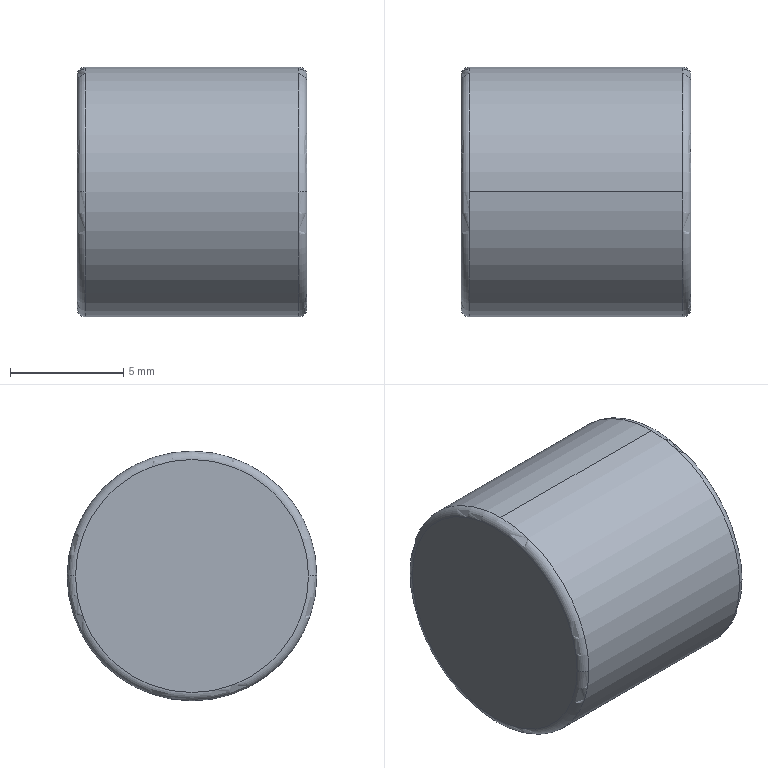Part | SolidWorks | features BaseBody 1 | 1 solid | 8 faces | box 10.125 x 11 x 11 mm | volume 960.225 mm3 | torus 4 | plane 2 | cylinder 2 | commonest cylinder face diameters 11 x2
STEP:
#1=CARTESIAN_POINT('',(-2090.144,780.437,-1577.624));
#2=VERTEX_POINT('',#1);
#3=CARTESIAN_POINT('',(-2090.144,790.7,-1577.624));
#4=VERTEX_POINT('',#3);
#5=CARTESIAN_POINT('',(-2090.144,785.569,-1577.624));
#6=DIRECTION('',(-1.,0.,0.));
#7=DIRECTION('',(0.,0.,1.));
#8=AXIS2_PLACEMENT_3D('',#5,#6,#7);
#9=CIRCLE('',#8,5.131);
#10=EDGE_CURVE('',#2,#4,#9,.T.);
#11=ORIENTED_EDGE('',*,*,#10,.T.);
#12=CARTESIAN_POINT('',(-2090.144,785.569,-1577.624));
#13=DIRECTION('',(-1.,0.,0.));
#14=DIRECTION('',(0.,1.,0.));
#15=AXIS2_PLACEMENT_3D('',#12,#13,#14);
#16=CIRCLE('',#15,5.131);
#17=EDGE_CURVE('',#4,#2,#16,.T.);
#18=ORIENTED_EDGE('',*,*,#17,.T.);
#19=EDGE_LOOP('',(#11,#18));
#20=FACE_OUTER_BOUND('',#19,.T.);
#21=CARTESIAN_POINT('',(-2090.144,779.924,-1583.231));
#22=DIRECTION('',(-1.,0.,0.));
#23=DIRECTION('',(0.,0.,1.));
#24=AXIS2_PLACEMENT_3D('',#21,#22,#23);
#25=PLANE('',#24);
#26=ADVANCED_FACE('',(#20),#25,.T.);
#27=CARTESIAN_POINT('',(-2089.775,780.069,-1577.624));
#28=VERTEX_POINT('',#27);
#29=CARTESIAN_POINT('',(-2089.775,780.437,-1577.624));
#30=DIRECTION('',(0.,0.,-1.));
#31=DIRECTION('',(0.,-1.,0.));
#32=AXIS2_PLACEMENT_3D('',#29,#30,#31);
#33=CIRCLE('',#32,0.3687);
#34=EDGE_CURVE('',#28,#2,#33,.T.);
#35=ORIENTED_EDGE('',*,*,#34,.T.);
#36=ORIENTED_EDGE('',*,*,#17,.F.);
#37=CARTESIAN_POINT('',(-2089.775,791.069,-1577.624));
#38=VERTEX_POINT('',#37);
#39=CARTESIAN_POINT('',(-2089.775,790.7,-1577.624));
#40=DIRECTION('',(0.,0.,-1.));
#41=DIRECTION('',(-1.,0.,0.));
#42=AXIS2_PLACEMENT_3D('',#39,#40,#41);
#43=CIRCLE('',#42,0.3687);
#44=EDGE_CURVE('',#4,#38,#43,.T.);
#45=ORIENTED_EDGE('',*,*,#44,.T.);
#46=CARTESIAN_POINT('',(-2089.775,785.569,-1583.124));
#47=VERTEX_POINT('',#46);
#48=CARTESIAN_POINT('',(-2089.775,785.569,-1577.624));
#49=DIRECTION('',(-1.,0.,0.));
#50=DIRECTION('',(0.,1.,0.));
#51=AXIS2_PLACEMENT_3D('',#48,#49,#50);
#52=CIRCLE('',#51,5.5);
#53=EDGE_CURVE('',#38,#47,#52,.T.);
#54=ORIENTED_EDGE('',*,*,#53,.T.);
#55=CARTESIAN_POINT('',(-2089.775,785.569,-1577.624));
#56=DIRECTION('',(-1.,0.,0.));
#57=DIRECTION('',(0.,0.,-1.));
#58=AXIS2_PLACEMENT_3D('',#55,#56,#57);
#59=CIRCLE('',#58,5.5);
#60=EDGE_CURVE('',#47,#28,#59,.T.);
#61=ORIENTED_EDGE('',*,*,#60,.T.);
#62=EDGE_LOOP('',(#35,#36,#45,#54,#61));
#63=FACE_OUTER_BOUND('',#62,.T.);
#64=CARTESIAN_POINT('',(-2089.775,785.569,-1577.624));
#65=DIRECTION('',(-1.,0.,0.));
#66=DIRECTION('',(0.,0.9962,0.08716));
#67=AXIS2_PLACEMENT_3D('',#64,#65,#66);
#68=TOROIDAL_SURFACE('',#67,5.131,0.3687);
#69=ADVANCED_FACE('',(#63),#68,.T.);
#70=CARTESIAN_POINT('',(-2080.388,785.569,-1572.124));
#71=VERTEX_POINT('',#70);
#72=CARTESIAN_POINT('',(-2089.775,785.569,-1572.124));
#73=VERTEX_POINT('',#72);
#74=CARTESIAN_POINT('',(-2080.388,785.569,-1572.124));
#75=DIRECTION('',(-1.,0.,0.));
#76=VECTOR('',#75,1000.);
#77=LINE('',#74,#76);
#78=EDGE_CURVE('',#71,#73,#77,.T.);
#79=ORIENTED_EDGE('',*,*,#78,.T.);
#80=CARTESIAN_POINT('',(-2089.775,785.569,-1577.624));
#81=DIRECTION('',(-1.,0.,0.));
#82=DIRECTION('',(0.,-1.,0.));
#83=AXIS2_PLACEMENT_3D('',#80,#81,#82);
#84=CIRCLE('',#83,5.5);
#85=EDGE_CURVE('',#28,#73,#84,.T.);
#86=ORIENTED_EDGE('',*,*,#85,.F.);
#87=ORIENTED_EDGE('',*,*,#60,.F.);
#88=CARTESIAN_POINT('',(-2080.388,785.569,-1583.124));
#89=VERTEX_POINT('',#88);
#90=CARTESIAN_POINT('',(-2089.775,785.569,-1583.124));
#91=DIRECTION('',(1.,0.,0.));
#92=VECTOR('',#91,1000.);
#93=LINE('',#90,#92);
#94=EDGE_CURVE('',#47,#89,#93,.T.);
#95=ORIENTED_EDGE('',*,*,#94,.T.);
#96=CARTESIAN_POINT('',(-2080.388,780.069,-1577.624));
#97=VERTEX_POINT('',#96);
#98=CARTESIAN_POINT('',(-2080.388,785.569,-1577.624));
#99=DIRECTION('',(-1.,0.,0.));
#100=DIRECTION('',(0.,0.,-1.));
#101=AXIS2_PLACEMENT_3D('',#98,#99,#100);
#102=CIRCLE('',#101,5.5);
#103=EDGE_CURVE('',#89,#97,#102,.T.);
#104=ORIENTED_EDGE('',*,*,#103,.T.);
#105=CARTESIAN_POINT('',(-2080.388,785.569,-1577.624));
#106=DIRECTION('',(-1.,0.,0.));
#107=DIRECTION('',(0.,-1.,0.));
#108=AXIS2_PLACEMENT_3D('',#105,#106,#107);
#109=CIRCLE('',#108,5.5);
#110=EDGE_CURVE('',#97,#71,#109,.T.);
#111=ORIENTED_EDGE('',*,*,#110,.T.);
#112=EDGE_LOOP('',(#79,#86,#87,#95,#104,#111));
#113=FACE_OUTER_BOUND('',#112,.T.);
#114=CARTESIAN_POINT('',(-2079.919,785.569,-1577.624));
#115=DIRECTION('',(1.,0.,0.));
#116=DIRECTION('',(0.,0.08716,0.9962));
#117=AXIS2_PLACEMENT_3D('',#114,#115,#116);
#118=CYLINDRICAL_SURFACE('',#117,5.5);
#119=ADVANCED_FACE('',(#113),#118,.T.);
#120=CARTESIAN_POINT('',(-2080.019,780.437,-1577.624));
#121=VERTEX_POINT('',#120);
#122=CARTESIAN_POINT('',(-2080.388,780.437,-1577.624));
#123=DIRECTION('',(0.,0.,-1.));
#124=DIRECTION('',(1.,0.,0.));
#125=AXIS2_PLACEMENT_3D('',#122,#123,#124);
#126=CIRCLE('',#125,0.3687);
#127=EDGE_CURVE('',#121,#97,#126,.T.);
#128=ORIENTED_EDGE('',*,*,#127,.T.);
#129=ORIENTED_EDGE('',*,*,#103,.F.);
#130=CARTESIAN_POINT('',(-2080.388,791.069,-1577.624));
#131=VERTEX_POINT('',#130);
#132=CARTESIAN_POINT('',(-2080.388,785.569,-1577.624));
#133=DIRECTION('',(-1.,0.,0.));
#134=DIRECTION('',(0.,1.,0.));
#135=AXIS2_PLACEMENT_3D('',#132,#133,#134);
#136=CIRCLE('',#135,5.5);
#137=EDGE_CURVE('',#131,#89,#136,.T.);
#138=ORIENTED_EDGE('',*,*,#137,.F.);
#139=CARTESIAN_POINT('',(-2080.019,790.7,-1577.624));
#140=VERTEX_POINT('',#139);
#141=CARTESIAN_POINT('',(-2080.388,790.7,-1577.624));
#142=DIRECTION('',(0.,0.,-1.));
#143=DIRECTION('',(0.,1.,0.));
#144=AXIS2_PLACEMENT_3D('',#141,#142,#143);
#145=CIRCLE('',#144,0.3687);
#146=EDGE_CURVE('',#131,#140,#145,.T.);
#147=ORIENTED_EDGE('',*,*,#146,.T.);
#148=CARTESIAN_POINT('',(-2080.019,785.569,-1577.624));
#149=DIRECTION('',(1.,0.,0.));
#150=DIRECTION('',(0.,-1.,0.));
#151=AXIS2_PLACEMENT_3D('',#148,#149,#150);
#152=CIRCLE('',#151,5.131);
#153=EDGE_CURVE('',#121,#140,#152,.T.);
#154=ORIENTED_EDGE('',*,*,#153,.F.);
#155=EDGE_LOOP('',(#128,#129,#138,#147,#154));
#156=FACE_OUTER_BOUND('',#155,.T.);
#157=CARTESIAN_POINT('',(-2080.388,785.569,-1577.624));
#158=DIRECTION('',(-1.,0.,0.));
#159=DIRECTION('',(0.,0.9962,0.08716));
#160=AXIS2_PLACEMENT_3D('',#157,#158,#159);
#161=TOROIDAL_SURFACE('',#160,5.131,0.3687);
#162=ADVANCED_FACE('',(#156),#161,.T.);
#163=CARTESIAN_POINT('',(-2080.019,785.569,-1577.624));
#164=DIRECTION('',(1.,0.,0.));
#165=DIRECTION('',(0.,1.,0.));
#166=AXIS2_PLACEMENT_3D('',#163,#164,#165);
#167=CIRCLE('',#166,5.131);
#168=EDGE_CURVE('',#140,#121,#167,.T.);
#169=ORIENTED_EDGE('',*,*,#168,.T.);
#170=ORIENTED_EDGE('',*,*,#153,.T.);
#171=EDGE_LOOP('',(#169,#170));
#172=FACE_OUTER_BOUND('',#171,.T.);
#173=CARTESIAN_POINT('',(-2080.019,779.924,-1571.98));
#174=DIRECTION('',(1.,0.,0.));
#175=DIRECTION('',(0.,1.,0.));
#176=AXIS2_PLACEMENT_3D('',#173,#174,#175);
#177=PLANE('',#176);
#178=ADVANCED_FACE('',(#172),#177,.T.);
#179=ORIENTED_EDGE('',*,*,#127,.F.);
#180=ORIENTED_EDGE('',*,*,#168,.F.);
#181=ORIENTED_EDGE('',*,*,#146,.F.);
#182=CARTESIAN_POINT('',(-2080.388,785.569,-1577.624));
#183=DIRECTION('',(-1.,0.,0.));
#184=DIRECTION('',(0.,0.,1.));
#185=AXIS2_PLACEMENT_3D('',#182,#183,#184);
#186=CIRCLE('',#185,5.5);
#187=EDGE_CURVE('',#71,#131,#186,.T.);
#188=ORIENTED_EDGE('',*,*,#187,.F.);
#189=ORIENTED_EDGE('',*,*,#110,.F.);
#190=EDGE_LOOP('',(#179,#180,#181,#188,#189));
#191=FACE_OUTER_BOUND('',#190,.T.);
#192=CARTESIAN_POINT('',(-2080.388,785.569,-1577.624));
#193=DIRECTION('',(-1.,0.,0.));
#194=DIRECTION('',(0.,-0.9962,-0.08716));
#195=AXIS2_PLACEMENT_3D('',#192,#193,#194);
#196=TOROIDAL_SURFACE('',#195,5.131,0.3687);
#197=ADVANCED_FACE('',(#191),#196,.T.);
#198=ORIENTED_EDGE('',*,*,#78,.F.);
#199=ORIENTED_EDGE('',*,*,#187,.T.);
#200=ORIENTED_EDGE('',*,*,#137,.T.);
#201=ORIENTED_EDGE('',*,*,#94,.F.);
#202=ORIENTED_EDGE('',*,*,#53,.F.);
#203=CARTESIAN_POINT('',(-2089.775,785.569,-1577.624));
#204=DIRECTION('',(-1.,0.,0.));
#205=DIRECTION('',(0.,0.,1.));
#206=AXIS2_PLACEMENT_3D('',#203,#204,#205);
#207=CIRCLE('',#206,5.5);
#208=EDGE_CURVE('',#73,#38,#207,.T.);
#209=ORIENTED_EDGE('',*,*,#208,.F.);
#210=EDGE_LOOP('',(#198,#199,#200,#201,#202,#209));
#211=FACE_OUTER_BOUND('',#210,.T.);
#212=CARTESIAN_POINT('',(-2079.919,785.569,-1577.624));
#213=DIRECTION('',(1.,0.,0.));
#214=DIRECTION('',(0.,-0.08716,-0.9962));
#215=AXIS2_PLACEMENT_3D('',#212,#213,#214);
#216=CYLINDRICAL_SURFACE('',#215,5.5);
#217=ADVANCED_FACE('',(#211),#216,.T.);
#218=ORIENTED_EDGE('',*,*,#34,.F.);
#219=ORIENTED_EDGE('',*,*,#85,.T.);
#220=ORIENTED_EDGE('',*,*,#208,.T.);
#221=ORIENTED_EDGE('',*,*,#44,.F.);
#222=ORIENTED_EDGE('',*,*,#10,.F.);
#223=EDGE_LOOP('',(#218,#219,#220,#221,#222));
#224=FACE_OUTER_BOUND('',#223,.T.);
#225=CARTESIAN_POINT('',(-2089.775,785.569,-1577.624));
#226=DIRECTION('',(-1.,0.,0.));
#227=DIRECTION('',(0.,-0.9962,-0.08716));
#228=AXIS2_PLACEMENT_3D('',#225,#226,#227);
#229=TOROIDAL_SURFACE('',#228,5.131,0.3687);
#230=ADVANCED_FACE('',(#224),#229,.T.);
#231=CLOSED_SHELL('',(#26,#69,#119,#162,#178,#197,#217,#230));
#232=MANIFOLD_SOLID_BREP('',#231);
#233=CARTESIAN_POINT('',(0.,0.,0.));
#234=DIRECTION('',(0.,0.,1.));
#235=DIRECTION('',(1.,0.,0.));
#236=AXIS2_PLACEMENT_3D('',#233,#234,#235);
#237=(LENGTH_UNIT()NAMED_UNIT(*)SI_UNIT(.MILLI.,.METRE.));
#238=UNCERTAINTY_MEASURE_WITH_UNIT(LENGTH_MEASURE(0.00001),#237,'','');
#239=(NAMED_UNIT(*)PLANE_ANGLE_UNIT()SI_UNIT($,.RADIAN.));
#240=(NAMED_UNIT(*)SI_UNIT($,.STERADIAN.)SOLID_ANGLE_UNIT());
#241=(GEOMETRIC_REPRESENTATION_CONTEXT(3)GLOBAL_UNCERTAINTY_ASSIGNED_CONTEXT((#238))GLOBAL_UNIT_ASSIGNED_CONTEXT((#237,#239,#240))REPRESENTATION_CONTEXT('',''));
#242=ADVANCED_BREP_SHAPE_REPRESENTATION('',(#232,#236),#241);